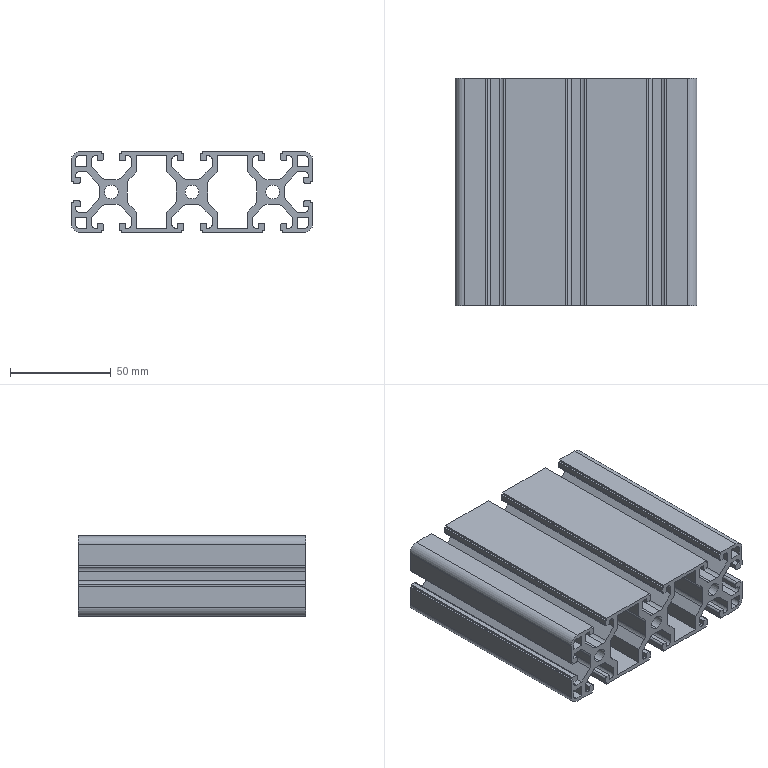Part | STEP file | Material transfer mechanism support_Default<machined> | 1 solid | 260 faces | box 120 x 112.995 x 40 mm | volume 180199 mm3 | plane 190 | cylinder 70 | commonest cylinder face diameters 6 x24 4 x20 2 x16 6.8 x6 9 x4